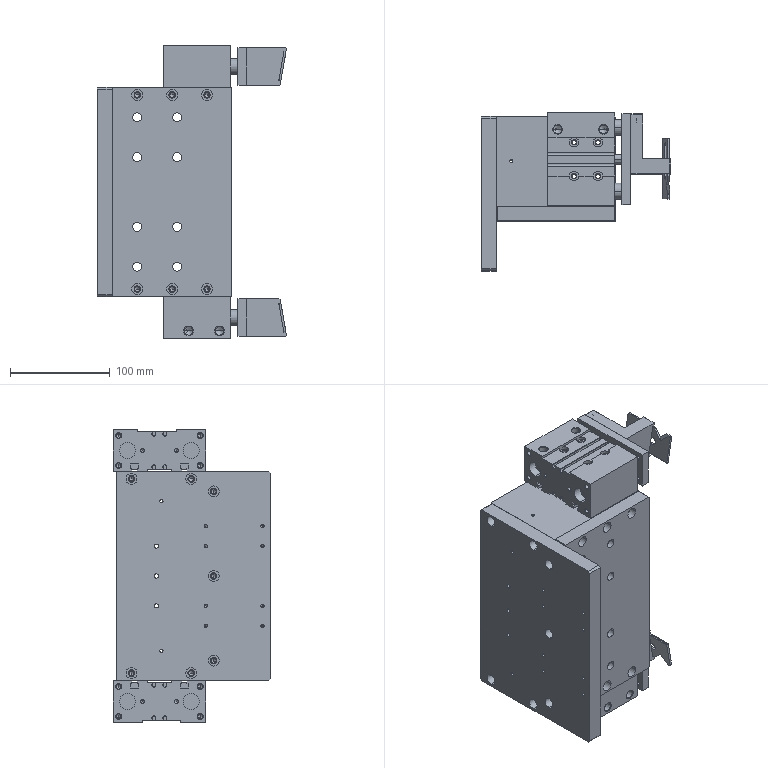Part | SolidWorks | 12 solids | 839 faces | box 189.85 x 158.5 x 294 mm | volume 1741491 mm3 | cylinder 374 | plane 275 | cone 190 | commonest cylinder face diameters 4.917 x48 4 x40 5 x38 6.6 x34 11 x34 3.3 x24